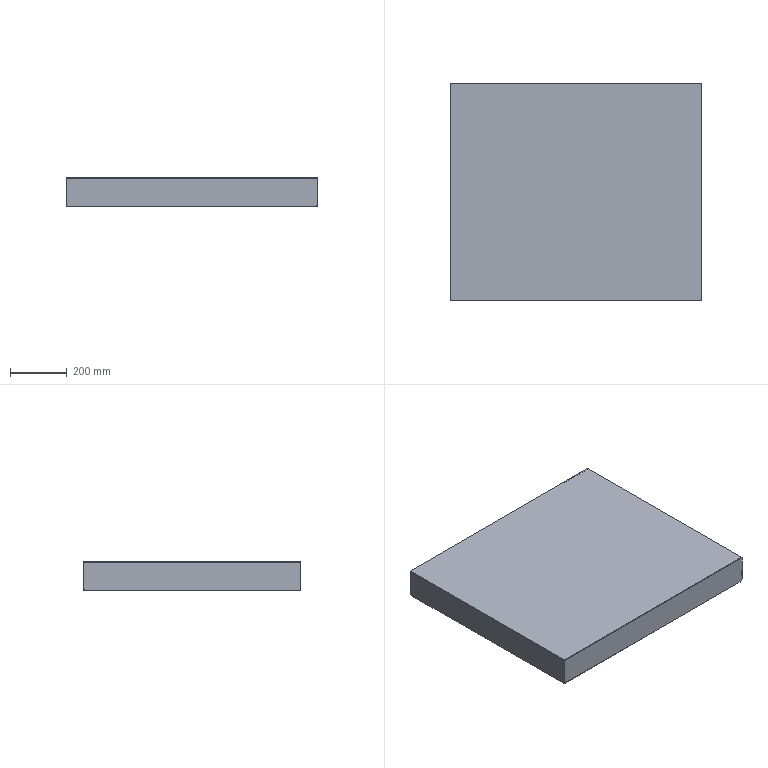Part | STEP file | PN_0047 checkered steel plate 3_Default<As Machined> | 3 solids | 23 faces | box 891 x 771 x 103 mm | volume 2594390 mm3 | plane 20 | cylinder 3 | commonest cylinder face diameters 20 x3
STEP:
#1=CARTESIAN_POINT('',(0.,0.,0.));
#2=DIRECTION('',(0.,0.,1.));
#3=DIRECTION('',(1.,0.,0.));
#4=AXIS2_PLACEMENT_3D('',#1,#2,#3);
#5=CARTESIAN_POINT('',(445.5,-385.5,0.));
#6=VERTEX_POINT('',#5);
#7=CARTESIAN_POINT('',(445.5,385.5,0.));
#8=VERTEX_POINT('',#7);
#9=CARTESIAN_POINT('',(445.5,385.5,0.));
#10=DIRECTION('',(0.,1.,0.));
#11=VECTOR('',#10,1.);
#12=LINE('',#9,#11);
#13=CARTESIAN_POINT('',(445.5,385.5,-3.));
#14=DIRECTION('',(1.,0.,0.));
#15=DIRECTION('',(0.,0.,-1.));
#16=AXIS2_PLACEMENT_3D('',#13,#14,#15);
#17=PLANE('',#16);
#18=CARTESIAN_POINT('',(-3.,0.));
#19=DIRECTION('',(0.,1.));
#20=VECTOR('',#19,1.);
#21=LINE('',#18,#20);
#22=(GEOMETRIC_REPRESENTATION_CONTEXT(2)PARAMETRIC_REPRESENTATION_CONTEXT()REPRESENTATION_CONTEXT('',''));
#23=DEFINITIONAL_REPRESENTATION('',(#21),#22);
#24=PCURVE('',#17,#23);
#25=CARTESIAN_POINT('',(0.,0.,0.));
#26=DIRECTION('',(0.,0.,1.));
#27=DIRECTION('',(1.,0.,0.));
#28=AXIS2_PLACEMENT_3D('',#25,#26,#27);
#29=PLANE('',#28);
#30=CARTESIAN_POINT('',(445.5,385.5));
#31=DIRECTION('',(0.,1.));
#32=VECTOR('',#31,1.);
#33=LINE('',#30,#32);
#34=(GEOMETRIC_REPRESENTATION_CONTEXT(2)PARAMETRIC_REPRESENTATION_CONTEXT()REPRESENTATION_CONTEXT('',''));
#35=DEFINITIONAL_REPRESENTATION('',(#33),#34);
#36=PCURVE('',#29,#35);
#37=SURFACE_CURVE('',#12,(#24,#36),.PCURVE_S1.);
#38=EDGE_CURVE('',#6,#8,#37,.T.);
#39=ORIENTED_EDGE('',*,*,#38,.F.);
#40=CARTESIAN_POINT('',(445.5,-385.5,-3.));
#41=VERTEX_POINT('',#40);
#42=CARTESIAN_POINT('',(445.5,-385.5,-3.));
#43=DIRECTION('',(0.,0.,1.));
#44=VECTOR('',#43,1.);
#45=LINE('',#42,#44);
#46=CARTESIAN_POINT('',(0.,-771.));
#47=DIRECTION('',(-1.,0.));
#48=VECTOR('',#47,1.);
#49=LINE('',#46,#48);
#50=(GEOMETRIC_REPRESENTATION_CONTEXT(2)PARAMETRIC_REPRESENTATION_CONTEXT()REPRESENTATION_CONTEXT('',''));
#51=DEFINITIONAL_REPRESENTATION('',(#49),#50);
#52=PCURVE('',#17,#51);
#53=CARTESIAN_POINT('',(-445.5,-385.5,-3.));
#54=DIRECTION('',(0.,-1.,0.));
#55=DIRECTION('',(0.,0.,-1.));
#56=AXIS2_PLACEMENT_3D('',#53,#54,#55);
#57=PLANE('',#56);
#58=CARTESIAN_POINT('',(0.,891.));
#59=DIRECTION('',(-1.,0.));
#60=VECTOR('',#59,1.);
#61=LINE('',#58,#60);
#62=(GEOMETRIC_REPRESENTATION_CONTEXT(2)PARAMETRIC_REPRESENTATION_CONTEXT()REPRESENTATION_CONTEXT('',''));
#63=DEFINITIONAL_REPRESENTATION('',(#61),#62);
#64=PCURVE('',#57,#63);
#65=SURFACE_CURVE('',#45,(#52,#64),.PCURVE_S1.);
#66=EDGE_CURVE('',#41,#6,#65,.T.);
#67=ORIENTED_EDGE('',*,*,#66,.F.);
#68=CARTESIAN_POINT('',(445.5,385.5,-3.));
#69=VERTEX_POINT('',#68);
#70=CARTESIAN_POINT('',(445.5,385.5,-3.));
#71=DIRECTION('',(0.,1.,0.));
#72=VECTOR('',#71,1.);
#73=LINE('',#70,#72);
#74=CARTESIAN_POINT('',(0.,0.));
#75=DIRECTION('',(0.,1.));
#76=VECTOR('',#75,1.);
#77=LINE('',#74,#76);
#78=(GEOMETRIC_REPRESENTATION_CONTEXT(2)PARAMETRIC_REPRESENTATION_CONTEXT()REPRESENTATION_CONTEXT('',''));
#79=DEFINITIONAL_REPRESENTATION('',(#77),#78);
#80=PCURVE('',#17,#79);
#81=CARTESIAN_POINT('',(0.,0.,-3.));
#82=DIRECTION('',(0.,0.,1.));
#83=DIRECTION('',(1.,0.,0.));
#84=AXIS2_PLACEMENT_3D('',#81,#82,#83);
#85=PLANE('',#84);
#86=CARTESIAN_POINT('',(445.5,385.5));
#87=DIRECTION('',(0.,1.));
#88=VECTOR('',#87,1.);
#89=LINE('',#86,#88);
#90=(GEOMETRIC_REPRESENTATION_CONTEXT(2)PARAMETRIC_REPRESENTATION_CONTEXT()REPRESENTATION_CONTEXT('',''));
#91=DEFINITIONAL_REPRESENTATION('',(#89),#90);
#92=PCURVE('',#85,#91);
#93=SURFACE_CURVE('',#73,(#80,#92),.PCURVE_S1.);
#94=EDGE_CURVE('',#41,#69,#93,.T.);
#95=ORIENTED_EDGE('',*,*,#94,.T.);
#96=CARTESIAN_POINT('',(445.5,385.5,-3.));
#97=DIRECTION('',(0.,0.,1.));
#98=VECTOR('',#97,1.);
#99=LINE('',#96,#98);
#100=CARTESIAN_POINT('',(0.,0.));
#101=DIRECTION('',(-1.,0.));
#102=VECTOR('',#101,1.);
#103=LINE('',#100,#102);
#104=(GEOMETRIC_REPRESENTATION_CONTEXT(2)PARAMETRIC_REPRESENTATION_CONTEXT()REPRESENTATION_CONTEXT('',''));
#105=DEFINITIONAL_REPRESENTATION('',(#103),#104);
#106=PCURVE('',#17,#105);
#107=CARTESIAN_POINT('',(-445.5,385.5,-3.));
#108=DIRECTION('',(0.,1.,0.));
#109=DIRECTION('',(0.,0.,1.));
#110=AXIS2_PLACEMENT_3D('',#107,#108,#109);
#111=PLANE('',#110);
#112=CARTESIAN_POINT('',(0.,891.));
#113=DIRECTION('',(1.,0.));
#114=VECTOR('',#113,1.);
#115=LINE('',#112,#114);
#116=(GEOMETRIC_REPRESENTATION_CONTEXT(2)PARAMETRIC_REPRESENTATION_CONTEXT()REPRESENTATION_CONTEXT('',''));
#117=DEFINITIONAL_REPRESENTATION('',(#115),#116);
#118=PCURVE('',#111,#117);
#119=SURFACE_CURVE('',#99,(#106,#118),.PCURVE_S1.);
#120=EDGE_CURVE('',#69,#8,#119,.T.);
#121=ORIENTED_EDGE('',*,*,#120,.T.);
#122=EDGE_LOOP('',(#39,#67,#95,#121));
#123=FACE_BOUND('',#122,.T.);
#124=ADVANCED_FACE('',(#123),#17,.T.);
#125=CARTESIAN_POINT('',(-445.5,-385.5,0.));
#126=VERTEX_POINT('',#125);
#127=CARTESIAN_POINT('',(-445.5,-385.5,0.));
#128=DIRECTION('',(1.,0.,0.));
#129=VECTOR('',#128,1.);
#130=LINE('',#127,#129);
#131=CARTESIAN_POINT('',(-3.,0.));
#132=DIRECTION('',(0.,1.));
#133=VECTOR('',#132,1.);
#134=LINE('',#131,#133);
#135=(GEOMETRIC_REPRESENTATION_CONTEXT(2)PARAMETRIC_REPRESENTATION_CONTEXT()REPRESENTATION_CONTEXT('',''));
#136=DEFINITIONAL_REPRESENTATION('',(#134),#135);
#137=PCURVE('',#57,#136);
#138=CARTESIAN_POINT('',(-445.5,-385.5));
#139=DIRECTION('',(1.,0.));
#140=VECTOR('',#139,1.);
#141=LINE('',#138,#140);
#142=(GEOMETRIC_REPRESENTATION_CONTEXT(2)PARAMETRIC_REPRESENTATION_CONTEXT()REPRESENTATION_CONTEXT('',''));
#143=DEFINITIONAL_REPRESENTATION('',(#141),#142);
#144=PCURVE('',#29,#143);
#145=SURFACE_CURVE('',#130,(#137,#144),.PCURVE_S1.);
#146=EDGE_CURVE('',#126,#6,#145,.T.);
#147=ORIENTED_EDGE('',*,*,#146,.F.);
#148=CARTESIAN_POINT('',(-445.5,-385.5,-3.));
#149=VERTEX_POINT('',#148);
#150=CARTESIAN_POINT('',(-445.5,-385.5,-3.));
#151=DIRECTION('',(0.,0.,1.));
#152=VECTOR('',#151,1.);
#153=LINE('',#150,#152);
#154=CARTESIAN_POINT('',(0.,0.));
#155=DIRECTION('',(-1.,0.));
#156=VECTOR('',#155,1.);
#157=LINE('',#154,#156);
#158=(GEOMETRIC_REPRESENTATION_CONTEXT(2)PARAMETRIC_REPRESENTATION_CONTEXT()REPRESENTATION_CONTEXT('',''));
#159=DEFINITIONAL_REPRESENTATION('',(#157),#158);
#160=PCURVE('',#57,#159);
#161=CARTESIAN_POINT('',(-445.5,385.5,-3.));
#162=DIRECTION('',(-1.,0.,0.));
#163=DIRECTION('',(0.,0.,1.));
#164=AXIS2_PLACEMENT_3D('',#161,#162,#163);
#165=PLANE('',#164);
#166=CARTESIAN_POINT('',(0.,-771.));
#167=DIRECTION('',(1.,0.));
#168=VECTOR('',#167,1.);
#169=LINE('',#166,#168);
#170=(GEOMETRIC_REPRESENTATION_CONTEXT(2)PARAMETRIC_REPRESENTATION_CONTEXT()REPRESENTATION_CONTEXT('',''));
#171=DEFINITIONAL_REPRESENTATION('',(#169),#170);
#172=PCURVE('',#165,#171);
#173=SURFACE_CURVE('',#153,(#160,#172),.PCURVE_S1.);
#174=EDGE_CURVE('',#149,#126,#173,.T.);
#175=ORIENTED_EDGE('',*,*,#174,.F.);
#176=CARTESIAN_POINT('',(-445.5,-385.5,-3.));
#177=DIRECTION('',(1.,0.,0.));
#178=VECTOR('',#177,1.);
#179=LINE('',#176,#178);
#180=CARTESIAN_POINT('',(0.,0.));
#181=DIRECTION('',(0.,1.));
#182=VECTOR('',#181,1.);
#183=LINE('',#180,#182);
#184=(GEOMETRIC_REPRESENTATION_CONTEXT(2)PARAMETRIC_REPRESENTATION_CONTEXT()REPRESENTATION_CONTEXT('',''));
#185=DEFINITIONAL_REPRESENTATION('',(#183),#184);
#186=PCURVE('',#57,#185);
#187=CARTESIAN_POINT('',(-445.5,-385.5));
#188=DIRECTION('',(1.,0.));
#189=VECTOR('',#188,1.);
#190=LINE('',#187,#189);
#191=(GEOMETRIC_REPRESENTATION_CONTEXT(2)PARAMETRIC_REPRESENTATION_CONTEXT()REPRESENTATION_CONTEXT('',''));
#192=DEFINITIONAL_REPRESENTATION('',(#190),#191);
#193=PCURVE('',#85,#192);
#194=SURFACE_CURVE('',#179,(#186,#193),.PCURVE_S1.);
#195=EDGE_CURVE('',#149,#41,#194,.T.);
#196=ORIENTED_EDGE('',*,*,#195,.T.);
#197=ORIENTED_EDGE('',*,*,#66,.T.);
#198=EDGE_LOOP('',(#147,#175,#196,#197));
#199=FACE_BOUND('',#198,.T.);
#200=ADVANCED_FACE('',(#199),#57,.T.);
#201=CARTESIAN_POINT('',(-445.5,385.5,0.));
#202=VERTEX_POINT('',#201);
#203=CARTESIAN_POINT('',(-445.5,385.5,0.));
#204=DIRECTION('',(0.,-1.,0.));
#205=VECTOR('',#204,1.);
#206=LINE('',#203,#205);
#207=CARTESIAN_POINT('',(3.,0.));
#208=DIRECTION('',(0.,-1.));
#209=VECTOR('',#208,1.);
#210=LINE('',#207,#209);
#211=(GEOMETRIC_REPRESENTATION_CONTEXT(2)PARAMETRIC_REPRESENTATION_CONTEXT()REPRESENTATION_CONTEXT('',''));
#212=DEFINITIONAL_REPRESENTATION('',(#210),#211);
#213=PCURVE('',#165,#212);
#214=CARTESIAN_POINT('',(-445.5,385.5));
#215=DIRECTION('',(0.,-1.));
#216=VECTOR('',#215,1.);
#217=LINE('',#214,#216);
#218=(GEOMETRIC_REPRESENTATION_CONTEXT(2)PARAMETRIC_REPRESENTATION_CONTEXT()REPRESENTATION_CONTEXT('',''));
#219=DEFINITIONAL_REPRESENTATION('',(#217),#218);
#220=PCURVE('',#29,#219);
#221=SURFACE_CURVE('',#206,(#213,#220),.PCURVE_S1.);
#222=EDGE_CURVE('',#202,#126,#221,.T.);
#223=ORIENTED_EDGE('',*,*,#222,.F.);
#224=CARTESIAN_POINT('',(-445.5,385.5,-3.));
#225=VERTEX_POINT('',#224);
#226=CARTESIAN_POINT('',(-445.5,385.5,-3.));
#227=DIRECTION('',(0.,0.,1.));
#228=VECTOR('',#227,1.);
#229=LINE('',#226,#228);
#230=CARTESIAN_POINT('',(0.,0.));
#231=DIRECTION('',(1.,0.));
#232=VECTOR('',#231,1.);
#233=LINE('',#230,#232);
#234=(GEOMETRIC_REPRESENTATION_CONTEXT(2)PARAMETRIC_REPRESENTATION_CONTEXT()REPRESENTATION_CONTEXT('',''));
#235=DEFINITIONAL_REPRESENTATION('',(#233),#234);
#236=PCURVE('',#165,#235);
#237=CARTESIAN_POINT('',(0.,0.));
#238=DIRECTION('',(1.,0.));
#239=VECTOR('',#238,1.);
#240=LINE('',#237,#239);
#241=(GEOMETRIC_REPRESENTATION_CONTEXT(2)PARAMETRIC_REPRESENTATION_CONTEXT()REPRESENTATION_CONTEXT('',''));
#242=DEFINITIONAL_REPRESENTATION('',(#240),#241);
#243=PCURVE('',#111,#242);
#244=SURFACE_CURVE('',#229,(#236,#243),.PCURVE_S1.);
#245=EDGE_CURVE('',#225,#202,#244,.T.);
#246=ORIENTED_EDGE('',*,*,#245,.F.);
#247=CARTESIAN_POINT('',(-445.5,385.5,-3.));
#248=DIRECTION('',(0.,-1.,0.));
#249=VECTOR('',#248,1.);
#250=LINE('',#247,#249);
#251=CARTESIAN_POINT('',(0.,0.));
#252=DIRECTION('',(0.,-1.));
#253=VECTOR('',#252,1.);
#254=LINE('',#251,#253);
#255=(GEOMETRIC_REPRESENTATION_CONTEXT(2)PARAMETRIC_REPRESENTATION_CONTEXT()REPRESENTATION_CONTEXT('',''));
#256=DEFINITIONAL_REPRESENTATION('',(#254),#255);
#257=PCURVE('',#165,#256);
#258=CARTESIAN_POINT('',(-445.5,385.5));
#259=DIRECTION('',(0.,-1.));
#260=VECTOR('',#259,1.);
#261=LINE('',#258,#260);
#262=(GEOMETRIC_REPRESENTATION_CONTEXT(2)PARAMETRIC_REPRESENTATION_CONTEXT()REPRESENTATION_CONTEXT('',''));
#263=DEFINITIONAL_REPRESENTATION('',(#261),#262);
#264=PCURVE('',#85,#263);
#265=SURFACE_CURVE('',#250,(#257,#264),.PCURVE_S1.);
#266=EDGE_CURVE('',#225,#149,#265,.T.);
#267=ORIENTED_EDGE('',*,*,#266,.T.);
#268=ORIENTED_EDGE('',*,*,#174,.T.);
#269=EDGE_LOOP('',(#223,#246,#267,#268));
#270=FACE_BOUND('',#269,.T.);
#271=ADVANCED_FACE('',(#270),#165,.T.);
#272=CARTESIAN_POINT('',(-445.5,385.5,0.));
#273=DIRECTION('',(-1.,0.,0.));
#274=VECTOR('',#273,1.);
#275=LINE('',#272,#274);
#276=CARTESIAN_POINT('',(3.,0.));
#277=DIRECTION('',(0.,-1.));
#278=VECTOR('',#277,1.);
#279=LINE('',#276,#278);
#280=(GEOMETRIC_REPRESENTATION_CONTEXT(2)PARAMETRIC_REPRESENTATION_CONTEXT()REPRESENTATION_CONTEXT('',''));
#281=DEFINITIONAL_REPRESENTATION('',(#279),#280);
#282=PCURVE('',#111,#281);
#283=CARTESIAN_POINT('',(-445.5,385.5));
#284=DIRECTION('',(-1.,0.));
#285=VECTOR('',#284,1.);
#286=LINE('',#283,#285);
#287=(GEOMETRIC_REPRESENTATION_CONTEXT(2)PARAMETRIC_REPRESENTATION_CONTEXT()REPRESENTATION_CONTEXT('',''));
#288=DEFINITIONAL_REPRESENTATION('',(#286),#287);
#289=PCURVE('',#29,#288);
#290=SURFACE_CURVE('',#275,(#282,#289),.PCURVE_S1.);
#291=EDGE_CURVE('',#8,#202,#290,.T.);
#292=ORIENTED_EDGE('',*,*,#291,.F.);
#293=ORIENTED_EDGE('',*,*,#120,.F.);
#294=CARTESIAN_POINT('',(-445.5,385.5,-3.));
#295=DIRECTION('',(-1.,0.,0.));
#296=VECTOR('',#295,1.);
#297=LINE('',#294,#296);
#298=CARTESIAN_POINT('',(0.,0.));
#299=DIRECTION('',(0.,-1.));
#300=VECTOR('',#299,1.);
#301=LINE('',#298,#300);
#302=(GEOMETRIC_REPRESENTATION_CONTEXT(2)PARAMETRIC_REPRESENTATION_CONTEXT()REPRESENTATION_CONTEXT('',''));
#303=DEFINITIONAL_REPRESENTATION('',(#301),#302);
#304=PCURVE('',#111,#303);
#305=CARTESIAN_POINT('',(-445.5,385.5));
#306=DIRECTION('',(-1.,0.));
#307=VECTOR('',#306,1.);
#308=LINE('',#305,#307);
#309=(GEOMETRIC_REPRESENTATION_CONTEXT(2)PARAMETRIC_REPRESENTATION_CONTEXT()REPRESENTATION_CONTEXT('',''));
#310=DEFINITIONAL_REPRESENTATION('',(#308),#309);
#311=PCURVE('',#85,#310);
#312=SURFACE_CURVE('',#297,(#304,#311),.PCURVE_S1.);
#313=EDGE_CURVE('',#69,#225,#312,.T.);
#314=ORIENTED_EDGE('',*,*,#313,.T.);
#315=ORIENTED_EDGE('',*,*,#245,.T.);
#316=EDGE_LOOP('',(#292,#293,#314,#315));
#317=FACE_BOUND('',#316,.T.);
#318=ADVANCED_FACE('',(#317),#111,.T.);
#319=ORIENTED_EDGE('',*,*,#94,.F.);
#320=ORIENTED_EDGE('',*,*,#195,.F.);
#321=ORIENTED_EDGE('',*,*,#266,.F.);
#322=ORIENTED_EDGE('',*,*,#313,.F.);
#323=EDGE_LOOP('',(#319,#320,#321,#322));
#324=FACE_BOUND('',#323,.T.);
#325=ADVANCED_FACE('',(#324),#85,.F.);
#326=ORIENTED_EDGE('',*,*,#38,.T.);
#327=ORIENTED_EDGE('',*,*,#291,.T.);
#328=ORIENTED_EDGE('',*,*,#222,.T.);
#329=ORIENTED_EDGE('',*,*,#146,.T.);
#330=EDGE_LOOP('',(#326,#327,#328,#329));
#331=FACE_BOUND('',#330,.T.);
#332=ADVANCED_FACE('',(#331),#29,.T.);
#333=CLOSED_SHELL('',(#124,#200,#271,#318,#325,#332));
#334=MANIFOLD_SOLID_BREP('',#333);
#335=CARTESIAN_POINT('',(-445.5,-385.5,-103.));
#336=VERTEX_POINT('',#335);
#337=CARTESIAN_POINT('',(435.5,-385.5,-103.));
#338=VERTEX_POINT('',#337);
#339=CARTESIAN_POINT('',(-445.5,-385.5,-103.));
#340=DIRECTION('',(1.,0.,0.));
#341=VECTOR('',#340,1.);
#342=LINE('',#339,#341);
#343=CARTESIAN_POINT('',(-445.5,-385.5,-103.));
#344=DIRECTION('',(0.,-1.,0.));
#345=DIRECTION('',(0.,0.,-1.));
#346=AXIS2_PLACEMENT_3D('',#343,#344,#345);
#347=PLANE('',#346);
#348=CARTESIAN_POINT('',(0.,0.));
#349=DIRECTION('',(0.,1.));
#350=VECTOR('',#349,1.);
#351=LINE('',#348,#350);
#352=(GEOMETRIC_REPRESENTATION_CONTEXT(2)PARAMETRIC_REPRESENTATION_CONTEXT()REPRESENTATION_CONTEXT('',''));
#353=DEFINITIONAL_REPRESENTATION('',(#351),#352);
#354=PCURVE('',#347,#353);
#355=CARTESIAN_POINT('',(0.,0.,-103.));
#356=DIRECTION('',(0.,0.,-1.));
#357=DIRECTION('',(-1.,0.,0.));
#358=AXIS2_PLACEMENT_3D('',#355,#356,#357);
#359=PLANE('',#358);
#360=CARTESIAN_POINT('',(445.5,-385.5));
#361=DIRECTION('',(-1.,0.));
#362=VECTOR('',#361,1.);
#363=LINE('',#360,#362);
#364=(GEOMETRIC_REPRESENTATION_CONTEXT(2)PARAMETRIC_REPRESENTATION_CONTEXT()REPRESENTATION_CONTEXT('',''));
#365=DEFINITIONAL_REPRESENTATION('',(#363),#364);
#366=PCURVE('',#359,#365);
#367=SURFACE_CURVE('',#342,(#354,#366),.PCURVE_S1.);
#368=EDGE_CURVE('',#336,#338,#367,.T.);
#369=ORIENTED_EDGE('',*,*,#368,.T.);
#370=CARTESIAN_POINT('',(445.5,-385.5,-93.));
#371=VERTEX_POINT('',#370);
#372=CARTESIAN_POINT('',(435.5,-385.5,-93.));
#373=DIRECTION('',(0.,-1.,0.));
#374=DIRECTION('',(0.,0.,-1.));
#375=AXIS2_PLACEMENT_3D('',#372,#373,#374);
#376=CIRCLE('',#375,10.);
#377=CARTESIAN_POINT('',(-10.,881.));
#378=DIRECTION('',(1.,0.));
#379=AXIS2_PLACEMENT_2D('',#377,#378);
#380=CIRCLE('',#379,10.);
#381=(GEOMETRIC_REPRESENTATION_CONTEXT(2)PARAMETRIC_REPRESENTATION_CONTEXT()REPRESENTATION_CONTEXT('',''));
#382=DEFINITIONAL_REPRESENTATION('',(#380),#381);
#383=PCURVE('',#347,#382);
#384=CARTESIAN_POINT('',(435.5,0.,-93.));
#385=DIRECTION('',(0.,1.,0.));
#386=DIRECTION('',(0.,0.,1.));
#387=AXIS2_PLACEMENT_3D('',#384,#385,#386);
#388=CYLINDRICAL_SURFACE('',#387,10.);
#389=CARTESIAN_POINT('',(3.142,-385.5));
#390=DIRECTION('',(-1.,0.));
#391=VECTOR('',#390,1.);
#392=LINE('',#389,#391);
#393=(GEOMETRIC_REPRESENTATION_CONTEXT(2)PARAMETRIC_REPRESENTATION_CONTEXT()REPRESENTATION_CONTEXT('',''));
#394=DEFINITIONAL_REPRESENTATION('',(#392),#393);
#395=PCURVE('',#388,#394);
#396=SURFACE_CURVE('',#376,(#383,#395),.PCURVE_S1.);
#397=EDGE_CURVE('',#338,#371,#396,.T.);
#398=ORIENTED_EDGE('',*,*,#397,.T.);
#399=CARTESIAN_POINT('',(445.5,-385.5,-3.));
#400=VERTEX_POINT('',#399);
#401=CARTESIAN_POINT('',(445.5,-385.5,-103.));
#402=DIRECTION('',(0.,0.,1.));
#403=VECTOR('',#402,1.);
#404=LINE('',#401,#403);
#405=CARTESIAN_POINT('',(0.,891.));
#406=DIRECTION('',(-1.,0.));
#407=VECTOR('',#406,1.);
#408=LINE('',#405,#407);
#409=(GEOMETRIC_REPRESENTATION_CONTEXT(2)PARAMETRIC_REPRESENTATION_CONTEXT()REPRESENTATION_CONTEXT('',''));
#410=DEFINITIONAL_REPRESENTATION('',(#408),#409);
#411=PCURVE('',#347,#410);
#412=CARTESIAN_POINT('',(445.5,-382.5,-103.));
#413=DIRECTION('',(-1.,0.,0.));
#414=DIRECTION('',(0.,0.,1.));
#415=AXIS2_PLACEMENT_3D('',#412,#413,#414);
#416=PLANE('',#415);
#417=CARTESIAN_POINT('',(0.,-3.));
#418=DIRECTION('',(1.,0.));
#419=VECTOR('',#418,1.);
#420=LINE('',#417,#419);
#421=(GEOMETRIC_REPRESENTATION_CONTEXT(2)PARAMETRIC_REPRESENTATION_CONTEXT()REPRESENTATION_CONTEXT('',''));
#422=DEFINITIONAL_REPRESENTATION('',(#420),#421);
#423=PCURVE('',#416,#422);
#424=SURFACE_CURVE('',#404,(#411,#423),.PCURVE_S1.);
#425=EDGE_CURVE('',#371,#400,#424,.T.);
#426=ORIENTED_EDGE('',*,*,#425,.T.);
#427=CARTESIAN_POINT('',(-445.5,-385.5,-3.));
#428=VERTEX_POINT('',#427);
#429=CARTESIAN_POINT('',(-445.5,-385.5,-3.));
#430=DIRECTION('',(1.,0.,0.));
#431=VECTOR('',#430,1.);
#432=LINE('',#429,#431);
#433=CARTESIAN_POINT('',(-100.,0.));
#434=DIRECTION('',(0.,1.));
#435=VECTOR('',#434,1.);
#436=LINE('',#433,#435);
#437=(GEOMETRIC_REPRESENTATION_CONTEXT(2)PARAMETRIC_REPRESENTATION_CONTEXT()REPRESENTATION_CONTEXT('',''));
#438=DEFINITIONAL_REPRESENTATION('',(#436),#437);
#439=PCURVE('',#347,#438);
#440=CARTESIAN_POINT('',(0.,0.,-3.));
#441=DIRECTION('',(0.,0.,-1.));
#442=DIRECTION('',(-1.,0.,0.));
#443=AXIS2_PLACEMENT_3D('',#440,#441,#442);
#444=PLANE('',#443);
#445=CARTESIAN_POINT('',(445.5,-385.5));
#446=DIRECTION('',(-1.,0.));
#447=VECTOR('',#446,1.);
#448=LINE('',#445,#447);
#449=(GEOMETRIC_REPRESENTATION_CONTEXT(2)PARAMETRIC_REPRESENTATION_CONTEXT()REPRESENTATION_CONTEXT('',''));
#450=DEFINITIONAL_REPRESENTATION('',(#448),#449);
#451=PCURVE('',#444,#450);
#452=SURFACE_CURVE('',#432,(#439,#451),.PCURVE_S1.);
#453=EDGE_CURVE('',#428,#400,#452,.T.);
#454=ORIENTED_EDGE('',*,*,#453,.F.);
#455=CARTESIAN_POINT('',(-445.5,-385.5,-103.));
#456=DIRECTION('',(0.,0.,1.));
#457=VECTOR('',#456,1.);
#458=LINE('',#455,#457);
#459=CARTESIAN_POINT('',(0.,0.));
#460=DIRECTION('',(-1.,0.));
#461=VECTOR('',#460,1.);
#462=LINE('',#459,#461);
#463=(GEOMETRIC_REPRESENTATION_CONTEXT(2)PARAMETRIC_REPRESENTATION_CONTEXT()REPRESENTATION_CONTEXT('',''));
#464=DEFINITIONAL_REPRESENTATION('',(#462),#463);
#465=PCURVE('',#347,#464);
#466=CARTESIAN_POINT('',(-445.5,385.5,-103.));
#467=DIRECTION('',(-1.,0.,0.));
#468=DIRECTION('',(0.,0.,1.));
#469=AXIS2_PLACEMENT_3D('',#466,#467,#468);
#470=PLANE('',#469);
#471=CARTESIAN_POINT('',(0.,-771.));
#472=DIRECTION('',(1.,0.));
#473=VECTOR('',#472,1.);
#474=LINE('',#471,#473);
#475=(GEOMETRIC_REPRESENTATION_CONTEXT(2)PARAMETRIC_REPRESENTATION_CONTEXT()REPRESENTATION_CONTEXT('',''));
#476=DEFINITIONAL_REPRESENTATION('',(#474),#475);
#477=PCURVE('',#470,#476);
#478=SURFACE_CURVE('',#458,(#465,#477),.PCURVE_S1.);
#479=EDGE_CURVE('',#336,#428,#478,.T.);
#480=ORIENTED_EDGE('',*,*,#479,.F.);
#481=EDGE_LOOP('',(#369,#398,#426,#454,#480));
#482=FACE_BOUND('',#481,.T.);
#483=ADVANCED_FACE('',(#482),#347,.T.);
#484=CARTESIAN_POINT('',(-445.5,385.5,-93.));
#485=VERTEX_POINT('',#484);
#486=CARTESIAN_POINT('',(-445.5,385.5,-3.));
#487=VERTEX_POINT('',#486);
#488=CARTESIAN_POINT('',(-445.5,385.5,-103.));
#489=DIRECTION('',(0.,0.,1.));
#490=VECTOR('',#489,1.);
#491=LINE('',#488,#490);
#492=CARTESIAN_POINT('',(0.,0.));
#493=DIRECTION('',(1.,0.));
#494=VECTOR('',#493,1.);
#495=LINE('',#492,#494);
#496=(GEOMETRIC_REPRESENTATION_CONTEXT(2)PARAMETRIC_REPRESENTATION_CONTEXT()REPRESENTATION_CONTEXT('',''));
#497=DEFINITIONAL_REPRESENTATION('',(#495),#496);
#498=PCURVE('',#470,#497);
#499=CARTESIAN_POINT('',(-445.5,385.5,-103.));
#500=DIRECTION('',(0.,-1.,0.));
#501=DIRECTION('',(0.,0.,-1.));
#502=AXIS2_PLACEMENT_3D('',#499,#500,#501);
#503=PLANE('',#502);
#504=CARTESIAN_POINT('',(0.,0.));
#505=DIRECTION('',(-1.,0.));
#506=VECTOR('',#505,1.);
#507=LINE('',#504,#506);
#508=(GEOMETRIC_REPRESENTATION_CONTEXT(2)PARAMETRIC_REPRESENTATION_CONTEXT()REPRESENTATION_CONTEXT('',''));
#509=DEFINITIONAL_REPRESENTATION('',(#507),#508);
#510=PCURVE('',#503,#509);
#511=SURFACE_CURVE('',#491,(#498,#510),.PCURVE_S1.);
#512=EDGE_CURVE('',#485,#487,#511,.T.);
#513=ORIENTED_EDGE('',*,*,#512,.F.);
#514=CARTESIAN_POINT('',(-445.5,375.5,-103.));
#515=VERTEX_POINT('',#514);
#516=CARTESIAN_POINT('',(-445.5,375.5,-93.));
#517=DIRECTION('',(-1.,0.,0.));
#518=DIRECTION('',(0.,0.,1.));
#519=AXIS2_PLACEMENT_3D('',#516,#517,#518);
#520=CIRCLE('',#519,10.);
#521=CARTESIAN_POINT('',(10.,-10.));
#522=DIRECTION('',(1.,0.));
#523=AXIS2_PLACEMENT_2D('',#521,#522);
#524=CIRCLE('',#523,10.);
#525=(GEOMETRIC_REPRESENTATION_CONTEXT(2)PARAMETRIC_REPRESENTATION_CONTEXT()REPRESENTATION_CONTEXT('',''));
#526=DEFINITIONAL_REPRESENTATION('',(#524),#525);
#527=PCURVE('',#470,#526);
#528=CARTESIAN_POINT('',(0.,375.5,-93.));
#529=DIRECTION('',(-1.,0.,0.));
#530=DIRECTION('',(0.,0.,1.));
#531=AXIS2_PLACEMENT_3D('',#528,#529,#530);
#532=CYLINDRICAL_SURFACE('',#531,10.);
#533=CARTESIAN_POINT('',(0.,445.5));
#534=DIRECTION('',(1.,0.));
#535=VECTOR('',#534,1.);
#536=LINE('',#533,#535);
#537=(GEOMETRIC_REPRESENTATION_CONTEXT(2)PARAMETRIC_REPRESENTATION_CONTEXT()REPRESENTATION_CONTEXT('',''));
#538=DEFINITIONAL_REPRESENTATION('',(#536),#537);
#539=PCURVE('',#532,#538);
#540=SURFACE_CURVE('',#520,(#527,#539),.PCURVE_S1.);
#541=EDGE_CURVE('',#485,#515,#540,.T.);
#542=ORIENTED_EDGE('',*,*,#541,.T.);
#543=CARTESIAN_POINT('',(-445.5,385.5,-103.));
#544=DIRECTION('',(0.,-1.,0.));
#545=VECTOR('',#544,1.);
#546=LINE('',#543,#545);
#547=CARTESIAN_POINT('',(0.,0.));
#548=DIRECTION('',(0.,-1.));
#549=VECTOR('',#548,1.);
#550=LINE('',#547,#549);
#551=(GEOMETRIC_REPRESENTATION_CONTEXT(2)PARAMETRIC_REPRESENTATION_CONTEXT()REPRESENTATION_CONTEXT('',''));
#552=DEFINITIONAL_REPRESENTATION('',(#550),#551);
#553=PCURVE('',#470,#552);
#554=CARTESIAN_POINT('',(445.5,385.5));
#555=DIRECTION('',(0.,-1.));
#556=VECTOR('',#555,1.);
#557=LINE('',#554,#556);
#558=(GEOMETRIC_REPRESENTATION_CONTEXT(2)PARAMETRIC_REPRESENTATION_CONTEXT()REPRESENTATION_CONTEXT('',''));
#559=DEFINITIONAL_REPRESENTATION('',(#557),#558);
#560=PCURVE('',#359,#559);
#561=SURFACE_CURVE('',#546,(#553,#560),.PCURVE_S1.);
#562=EDGE_CURVE('',#515,#336,#561,.T.);
#563=ORIENTED_EDGE('',*,*,#562,.T.);
#564=ORIENTED_EDGE('',*,*,#479,.T.);
#565=CARTESIAN_POINT('',(-445.5,385.5,-3.));
#566=DIRECTION('',(0.,-1.,0.));
#567=VECTOR('',#566,1.);
#568=LINE('',#565,#567);
#569=CARTESIAN_POINT('',(100.,0.));
#570=DIRECTION('',(0.,-1.));
#571=VECTOR('',#570,1.);
#572=LINE('',#569,#571);
#573=(GEOMETRIC_REPRESENTATION_CONTEXT(2)PARAMETRIC_REPRESENTATION_CONTEXT()REPRESENTATION_CONTEXT('',''));
#574=DEFINITIONAL_REPRESENTATION('',(#572),#573);
#575=PCURVE('',#470,#574);
#576=CARTESIAN_POINT('',(445.5,385.5));
#577=DIRECTION('',(0.,-1.));
#578=VECTOR('',#577,1.);
#579=LINE('',#576,#578);
#580=(GEOMETRIC_REPRESENTATION_CONTEXT(2)PARAMETRIC_REPRESENTATION_CONTEXT()REPRESENTATION_CONTEXT('',''));
#581=DEFINITIONAL_REPRESENTATION('',(#579),#580);
#582=PCURVE('',#444,#581);
#583=SURFACE_CURVE('',#568,(#575,#582),.PCURVE_S1.);
#584=EDGE_CURVE('',#487,#428,#583,.T.);
#585=ORIENTED_EDGE('',*,*,#584,.F.);
#586=EDGE_LOOP('',(#513,#542,#563,#564,#585));
#587=FACE_BOUND('',#586,.T.);
#588=ADVANCED_FACE('',(#587),#470,.T.);
#589=CARTESIAN_POINT('',(-442.5,385.5,-93.));
#590=VERTEX_POINT('',#589);
#591=CARTESIAN_POINT('',(-442.5,385.5,-3.));
#592=VERTEX_POINT('',#591);
#593=CARTESIAN_POINT('',(-442.5,385.5,-103.));
#594=DIRECTION('',(0.,0.,1.));
#595=VECTOR('',#594,1.);
#596=LINE('',#593,#595);
#597=CARTESIAN_POINT('',(0.,3.));
#598=DIRECTION('',(-1.,0.));
#599=VECTOR('',#598,1.);
#600=LINE('',#597,#599);
#601=(GEOMETRIC_REPRESENTATION_CONTEXT(2)PARAMETRIC_REPRESENTATION_CONTEXT()REPRESENTATION_CONTEXT('',''));
#602=DEFINITIONAL_REPRESENTATION('',(#600),#601);
#603=PCURVE('',#503,#602);
#604=CARTESIAN_POINT('',(-442.5,385.5,-103.));
#605=DIRECTION('',(-1.,0.,0.));
#606=DIRECTION('',(0.,0.,1.));
#607=AXIS2_PLACEMENT_3D('',#604,#605,#606);
#608=PLANE('',#607);
#609=CARTESIAN_POINT('',(0.,0.));
#610=DIRECTION('',(1.,0.));
#611=VECTOR('',#610,1.);
#612=LINE('',#609,#611);
#613=(GEOMETRIC_REPRESENTATION_CONTEXT(2)PARAMETRIC_REPRESENTATION_CONTEXT()REPRESENTATION_CONTEXT('',''));
#614=DEFINITIONAL_REPRESENTATION('',(#612),#613);
#615=PCURVE('',#608,#614);
#616=SURFACE_CURVE('',#596,(#603,#615),.PCURVE_S1.);
#617=EDGE_CURVE('',#590,#592,#616,.T.);
#618=ORIENTED_EDGE('',*,*,#617,.F.);
#619=CARTESIAN_POINT('',(-445.5,385.5,-93.));
#620=DIRECTION('',(-1.,0.,0.));
#621=VECTOR('',#620,1.);
#622=LINE('',#619,#621);
#623=CARTESIAN_POINT('',(-10.,0.));
#624=DIRECTION('',(0.,-1.));
#625=VECTOR('',#624,1.);
#626=LINE('',#623,#625);
#627=(GEOMETRIC_REPRESENTATION_CONTEXT(2)PARAMETRIC_REPRESENTATION_CONTEXT()REPRESENTATION_CONTEXT('',''));
#628=DEFINITIONAL_REPRESENTATION('',(#626),#627);
#629=PCURVE('',#503,#628);
#630=CARTESIAN_POINT('',(1.571,445.5));
#631=DIRECTION('',(0.,1.));
#632=VECTOR('',#631,1.);
#633=LINE('',#630,#632);
#634=(GEOMETRIC_REPRESENTATION_CONTEXT(2)PARAMETRIC_REPRESENTATION_CONTEXT()REPRESENTATION_CONTEXT('',''));
#635=DEFINITIONAL_REPRESENTATION('',(#633),#634);
#636=PCURVE('',#532,#635);
#637=SURFACE_CURVE('',#622,(#629,#636),.PCURVE_S1.);
#638=EDGE_CURVE('',#590,#485,#637,.T.);
#639=ORIENTED_EDGE('',*,*,#638,.T.);
#640=ORIENTED_EDGE('',*,*,#512,.T.);
#641=CARTESIAN_POINT('',(-445.5,385.5,-3.));
#642=DIRECTION('',(1.,0.,0.));
#643=VECTOR('',#642,1.);
#644=LINE('',#641,#643);
#645=CARTESIAN_POINT('',(-100.,0.));
#646=DIRECTION('',(0.,1.));
#647=VECTOR('',#646,1.);
#648=LINE('',#645,#647);
#649=(GEOMETRIC_REPRESENTATION_CONTEXT(2)PARAMETRIC_REPRESENTATION_CONTEXT()REPRESENTATION_CONTEXT('',''));
#650=DEFINITIONAL_REPRESENTATION('',(#648),#649);
#651=PCURVE('',#503,#650);
#652=CARTESIAN_POINT('',(445.5,385.5));
#653=DIRECTION('',(-1.,0.));
#654=VECTOR('',#653,1.);
#655=LINE('',#652,#654);
#656=(GEOMETRIC_REPRESENTATION_CONTEXT(2)PARAMETRIC_REPRESENTATION_CONTEXT()REPRESENTATION_CONTEXT('',''));
#657=DEFINITIONAL_REPRESENTATION('',(#655),#656);
#658=PCURVE('',#444,#657);
#659=SURFACE_CURVE('',#644,(#651,#658),.PCURVE_S1.);
#660=EDGE_CURVE('',#487,#592,#659,.T.);
#661=ORIENTED_EDGE('',*,*,#660,.T.);
#662=EDGE_LOOP('',(#618,#639,#640,#661));
#663=FACE_BOUND('',#662,.T.);
#664=ADVANCED_FACE('',(#663),#503,.F.);
#665=CARTESIAN_POINT('',(-442.5,375.5,-103.));
#666=VERTEX_POINT('',#665);
#667=CARTESIAN_POINT('',(-442.5,-382.5,-103.));
#668=VERTEX_POINT('',#667);
#669=CARTESIAN_POINT('',(-442.5,385.5,-103.));
#670=DIRECTION('',(0.,-1.,0.));
#671=VECTOR('',#670,1.);
#672=LINE('',#669,#671);
#673=CARTESIAN_POINT('',(0.,0.));
#674=DIRECTION('',(0.,-1.));
#675=VECTOR('',#674,1.);
#676=LINE('',#673,#675);
#677=(GEOMETRIC_REPRESENTATION_CONTEXT(2)PARAMETRIC_REPRESENTATION_CONTEXT()REPRESENTATION_CONTEXT('',''));
#678=DEFINITIONAL_REPRESENTATION('',(#676),#677);
#679=PCURVE('',#608,#678);
#680=CARTESIAN_POINT('',(442.5,385.5));
#681=DIRECTION('',(0.,-1.));
#682=VECTOR('',#681,1.);
#683=LINE('',#680,#682);
#684=(GEOMETRIC_REPRESENTATION_CONTEXT(2)PARAMETRIC_REPRESENTATION_CONTEXT()REPRESENTATION_CONTEXT('',''));
#685=DEFINITIONAL_REPRESENTATION('',(#683),#684);
#686=PCURVE('',#359,#685);
#687=SURFACE_CURVE('',#672,(#679,#686),.PCURVE_S1.);
#688=EDGE_CURVE('',#666,#668,#687,.T.);
#689=ORIENTED_EDGE('',*,*,#688,.F.);
#690=CARTESIAN_POINT('',(-442.5,375.5,-93.));
#691=DIRECTION('',(1.,0.,0.));
#692=DIRECTION('',(0.,0.,1.));
#693=AXIS2_PLACEMENT_3D('',#690,#691,#692);
#694=CIRCLE('',#693,10.);
#695=CARTESIAN_POINT('',(20.,-10.));
#696=CARTESIAN_POINT('',(20.,-27.321));
#697=CARTESIAN_POINT('',(5.,-18.66));
#698=CARTESIAN_POINT('',(-10.,-10.));
#699=CARTESIAN_POINT('',(5.,-1.34));
#700=CARTESIAN_POINT('',(20.,7.321));
#701=CARTESIAN_POINT('',(20.,-10.));
#702=(BOUNDED_CURVE()B_SPLINE_CURVE(2,(#695,#696,#697,#698,#699,#700,#701),.UNSPECIFIED.,.T.,.F.)B_SPLINE_CURVE_WITH_KNOTS((1,2,2,2,2,1),(-2.094,0.,2.094,4.189,6.283,8.378),.UNSPECIFIED.)CURVE()GEOMETRIC_REPRESENTATION_ITEM()RATIONAL_B_SPLINE_CURVE((1.,0.5,1.,0.5,1.,0.5,1.))REPRESENTATION_ITEM(''));
#703=(GEOMETRIC_REPRESENTATION_CONTEXT(2)PARAMETRIC_REPRESENTATION_CONTEXT()REPRESENTATION_CONTEXT('',''));
#704=DEFINITIONAL_REPRESENTATION('',(#702),#703);
#705=PCURVE('',#608,#704);
#706=CARTESIAN_POINT('',(6.283,442.5));
#707=DIRECTION('',(-1.,0.));
#708=VECTOR('',#707,1.);
#709=LINE('',#706,#708);
#710=(GEOMETRIC_REPRESENTATION_CONTEXT(2)PARAMETRIC_REPRESENTATION_CONTEXT()REPRESENTATION_CONTEXT('',''));
#711=DEFINITIONAL_REPRESENTATION('',(#709),#710);
#712=PCURVE('',#532,#711);
#713=SURFACE_CURVE('',#694,(#705,#712),.PCURVE_S1.);
#714=EDGE_CURVE('',#666,#590,#713,.T.);
#715=ORIENTED_EDGE('',*,*,#714,.T.);
#716=ORIENTED_EDGE('',*,*,#617,.T.);
#717=CARTESIAN_POINT('',(-442.5,-382.5,-3.));
#718=VERTEX_POINT('',#717);
#719=CARTESIAN_POINT('',(-442.5,385.5,-3.));
#720=DIRECTION('',(0.,-1.,0.));
#721=VECTOR('',#720,1.);
#722=LINE('',#719,#721);
#723=CARTESIAN_POINT('',(100.,0.));
#724=DIRECTION('',(0.,-1.));
#725=VECTOR('',#724,1.);
#726=LINE('',#723,#725);
#727=(GEOMETRIC_REPRESENTATION_CONTEXT(2)PARAMETRIC_REPRESENTATION_CONTEXT()REPRESENTATION_CONTEXT('',''));
#728=DEFINITIONAL_REPRESENTATION('',(#726),#727);
#729=PCURVE('',#608,#728);
#730=CARTESIAN_POINT('',(442.5,385.5));
#731=DIRECTION('',(0.,-1.));
#732=VECTOR('',#731,1.);
#733=LINE('',#730,#732);
#734=(GEOMETRIC_REPRESENTATION_CONTEXT(2)PARAMETRIC_REPRESENTATION_CONTEXT()REPRESENTATION_CONTEXT('',''));
#735=DEFINITIONAL_REPRESENTATION('',(#733),#734);
#736=PCURVE('',#444,#735);
#737=SURFACE_CURVE('',#722,(#729,#736),.PCURVE_S1.);
#738=EDGE_CURVE('',#592,#718,#737,.T.);
#739=ORIENTED_EDGE('',*,*,#738,.T.);
#740=CARTESIAN_POINT('',(-442.5,-382.5,-103.));
#741=DIRECTION('',(0.,0.,1.));
#742=VECTOR('',#741,1.);
#743=LINE('',#740,#742);
#744=CARTESIAN_POINT('',(0.,-768.));
#745=DIRECTION('',(1.,0.));
#746=VECTOR('',#745,1.);
#747=LINE('',#744,#746);
#748=(GEOMETRIC_REPRESENTATION_CONTEXT(2)PARAMETRIC_REPRESENTATION_CONTEXT()REPRESENTATION_CONTEXT('',''));
#749=DEFINITIONAL_REPRESENTATION('',(#747),#748);
#750=PCURVE('',#608,#749);
#751=CARTESIAN_POINT('',(-445.5,-382.5,-103.));
#752=DIRECTION('',(0.,-1.,0.));
#753=DIRECTION('',(0.,0.,-1.));
#754=AXIS2_PLACEMENT_3D('',#751,#752,#753);
#755=PLANE('',#754);
#756=CARTESIAN_POINT('',(0.,3.));
#757=DIRECTION('',(-1.,0.));
#758=VECTOR('',#757,1.);
#759=LINE('',#756,#758);
#760=(GEOMETRIC_REPRESENTATION_CONTEXT(2)PARAMETRIC_REPRESENTATION_CONTEXT()REPRESENTATION_CONTEXT('',''));
#761=DEFINITIONAL_REPRESENTATION('',(#759),#760);
#762=PCURVE('',#755,#761);
#763=SURFACE_CURVE('',#743,(#750,#762),.PCURVE_S1.);
#764=EDGE_CURVE('',#668,#718,#763,.T.);
#765=ORIENTED_EDGE('',*,*,#764,.F.);
#766=EDGE_LOOP('',(#689,#715,#716,#739,#765));
#767=FACE_BOUND('',#766,.T.);
#768=ADVANCED_FACE('',(#767),#608,.F.);
#769=CARTESIAN_POINT('',(445.5,-382.5,-93.));
#770=VERTEX_POINT('',#769);
#771=CARTESIAN_POINT('',(445.5,-382.5,-3.));
#772=VERTEX_POINT('',#771);
#773=CARTESIAN_POINT('',(445.5,-382.5,-103.));
#774=DIRECTION('',(0.,0.,1.));
#775=VECTOR('',#774,1.);
#776=LINE('',#773,#775);
#777=CARTESIAN_POINT('',(0.,891.));
#778=DIRECTION('',(-1.,0.));
#779=VECTOR('',#778,1.);
#780=LINE('',#777,#779);
#781=(GEOMETRIC_REPRESENTATION_CONTEXT(2)PARAMETRIC_REPRESENTATION_CONTEXT()REPRESENTATION_CONTEXT('',''));
#782=DEFINITIONAL_REPRESENTATION('',(#780),#781);
#783=PCURVE('',#755,#782);
#784=CARTESIAN_POINT('',(0.,0.));
#785=DIRECTION('',(1.,0.));
#786=VECTOR('',#785,1.);
#787=LINE('',#784,#786);
#788=(GEOMETRIC_REPRESENTATION_CONTEXT(2)PARAMETRIC_REPRESENTATION_CONTEXT()REPRESENTATION_CONTEXT('',''));
#789=DEFINITIONAL_REPRESENTATION('',(#787),#788);
#790=PCURVE('',#416,#789);
#791=SURFACE_CURVE('',#776,(#783,#790),.PCURVE_S1.);
#792=EDGE_CURVE('',#770,#772,#791,.T.);
#793=ORIENTED_EDGE('',*,*,#792,.F.);
#794=CARTESIAN_POINT('',(435.5,-382.5,-103.));
#795=VERTEX_POINT('',#794);
#796=CARTESIAN_POINT('',(435.5,-382.5,-93.));
#797=DIRECTION('',(0.,1.,0.));
#798=DIRECTION('',(0.,0.,-1.));
#799=AXIS2_PLACEMENT_3D('',#796,#797,#798);
#800=CIRCLE('',#799,10.);
#801=CARTESIAN_POINT('',(0.,881.));
#802=CARTESIAN_POINT('',(0.,863.679));
#803=CARTESIAN_POINT('',(-15.,872.34));
#804=CARTESIAN_POINT('',(-30.,881.));
#805=CARTESIAN_POINT('',(-15.,889.66));
#806=CARTESIAN_POINT('',(0.,898.321));
#807=CARTESIAN_POINT('',(0.,881.));
#808=(BOUNDED_CURVE()B_SPLINE_CURVE(2,(#801,#802,#803,#804,#805,#806,#807),.UNSPECIFIED.,.T.,.F.)B_SPLINE_CURVE_WITH_KNOTS((1,2,2,2,2,1),(-2.094,0.,2.094,4.189,6.283,8.378),.UNSPECIFIED.)CURVE()GEOMETRIC_REPRESENTATION_ITEM()RATIONAL_B_SPLINE_CURVE((1.,0.5,1.,0.5,1.,0.5,1.))REPRESENTATION_ITEM(''));
#809=(GEOMETRIC_REPRESENTATION_CONTEXT(2)PARAMETRIC_REPRESENTATION_CONTEXT()REPRESENTATION_CONTEXT('',''));
#810=DEFINITIONAL_REPRESENTATION('',(#808),#809);
#811=PCURVE('',#755,#810);
#812=CARTESIAN_POINT('',(-3.142,-382.5));
#813=DIRECTION('',(1.,0.));
#814=VECTOR('',#813,1.);
#815=LINE('',#812,#814);
#816=(GEOMETRIC_REPRESENTATION_CONTEXT(2)PARAMETRIC_REPRESENTATION_CONTEXT()REPRESENTATION_CONTEXT('',''));
#817=DEFINITIONAL_REPRESENTATION('',(#815),#816);
#818=PCURVE('',#388,#817);
#819=SURFACE_CURVE('',#800,(#811,#818),.PCURVE_S1.);
#820=EDGE_CURVE('',#770,#795,#819,.T.);
#821=ORIENTED_EDGE('',*,*,#820,.T.);
#822=CARTESIAN_POINT('',(-445.5,-382.5,-103.));
#823=DIRECTION('',(1.,0.,0.));
#824=VECTOR('',#823,1.);
#825=LINE('',#822,#824);
#826=CARTESIAN_POINT('',(0.,0.));
#827=DIRECTION('',(0.,1.));
#828=VECTOR('',#827,1.);
#829=LINE('',#826,#828);
#830=(GEOMETRIC_REPRESENTATION_CONTEXT(2)PARAMETRIC_REPRESENTATION_CONTEXT()REPRESENTATION_CONTEXT('',''));
#831=DEFINITIONAL_REPRESENTATION('',(#829),#830);
#832=PCURVE('',#755,#831);
#833=CARTESIAN_POINT('',(445.5,-382.5));
#834=DIRECTION('',(-1.,0.));
#835=VECTOR('',#834,1.);
#836=LINE('',#833,#835);
#837=(GEOMETRIC_REPRESENTATION_CONTEXT(2)PARAMETRIC_REPRESENTATION_CONTEXT()REPRESENTATION_CONTEXT('',''));
#838=DEFINITIONAL_REPRESENTATION('',(#836),#837);
#839=PCURVE('',#359,#838);
#840=SURFACE_CURVE('',#825,(#832,#839),.PCURVE_S1.);
#841=EDGE_CURVE('',#668,#795,#840,.T.);
#842=ORIENTED_EDGE('',*,*,#841,.F.);
#843=ORIENTED_EDGE('',*,*,#764,.T.);
#844=CARTESIAN_POINT('',(-445.5,-382.5,-3.));
#845=DIRECTION('',(1.,0.,0.));
#846=VECTOR('',#845,1.);
#847=LINE('',#844,#846);
#848=CARTESIAN_POINT('',(-100.,0.));
#849=DIRECTION('',(0.,1.));
#850=VECTOR('',#849,1.);
#851=LINE('',#848,#850);
#852=(GEOMETRIC_REPRESENTATION_CONTEXT(2)PARAMETRIC_REPRESENTATION_CONTEXT()REPRESENTATION_CONTEXT('',''));
#853=DEFINITIONAL_REPRESENTATION('',(#851),#852);
#854=PCURVE('',#755,#853);
#855=CARTESIAN_POINT('',(445.5,-382.5));
#856=DIRECTION('',(-1.,0.));
#857=VECTOR('',#856,1.);
#858=LINE('',#855,#857);
#859=(GEOMETRIC_REPRESENTATION_CONTEXT(2)PARAMETRIC_REPRESENTATION_CONTEXT()REPRESENTATION_CONTEXT('',''));
#860=DEFINITIONAL_REPRESENTATION('',(#858),#859);
#861=PCURVE('',#444,#860);
#862=SURFACE_CURVE('',#847,(#854,#861),.PCURVE_S1.);
#863=EDGE_CURVE('',#718,#772,#862,.T.);
#864=ORIENTED_EDGE('',*,*,#863,.T.);
#865=EDGE_LOOP('',(#793,#821,#842,#843,#864));
#866=FACE_BOUND('',#865,.T.);
#867=ADVANCED_FACE('',(#866),#755,.F.);
#868=ORIENTED_EDGE('',*,*,#425,.F.);
#869=CARTESIAN_POINT('',(445.5,-382.5,-93.));
#870=DIRECTION('',(0.,1.,0.));
#871=VECTOR('',#870,1.);
#872=LINE('',#869,#871);
#873=CARTESIAN_POINT('',(10.,0.));
#874=DIRECTION('',(0.,1.));
#875=VECTOR('',#874,1.);
#876=LINE('',#873,#875);
#877=(GEOMETRIC_REPRESENTATION_CONTEXT(2)PARAMETRIC_REPRESENTATION_CONTEXT()REPRESENTATION_CONTEXT('',''));
#878=DEFINITIONAL_REPRESENTATION('',(#876),#877);
#879=PCURVE('',#416,#878);
#880=CARTESIAN_POINT('',(1.571,-382.5));
#881=DIRECTION('',(0.,1.));
#882=VECTOR('',#881,1.);
#883=LINE('',#880,#882);
#884=(GEOMETRIC_REPRESENTATION_CONTEXT(2)PARAMETRIC_REPRESENTATION_CONTEXT()REPRESENTATION_CONTEXT('',''));
#885=DEFINITIONAL_REPRESENTATION('',(#883),#884);
#886=PCURVE('',#388,#885);
#887=SURFACE_CURVE('',#872,(#879,#886),.PCURVE_S1.);
#888=EDGE_CURVE('',#371,#770,#887,.T.);
#889=ORIENTED_EDGE('',*,*,#888,.T.);
#890=ORIENTED_EDGE('',*,*,#792,.T.);
#891=CARTESIAN_POINT('',(445.5,-382.5,-3.));
#892=DIRECTION('',(0.,-1.,0.));
#893=VECTOR('',#892,1.);
#894=LINE('',#891,#893);
#895=CARTESIAN_POINT('',(100.,0.));
#896=DIRECTION('',(0.,-1.));
#897=VECTOR('',#896,1.);
#898=LINE('',#895,#897);
#899=(GEOMETRIC_REPRESENTATION_CONTEXT(2)PARAMETRIC_REPRESENTATION_CONTEXT()REPRESENTATION_CONTEXT('',''));
#900=DEFINITIONAL_REPRESENTATION('',(#898),#899);
#901=PCURVE('',#416,#900);
#902=CARTESIAN_POINT('',(-445.5,-382.5));
#903=DIRECTION('',(0.,-1.));
#904=VECTOR('',#903,1.);
#905=LINE('',#902,#904);
#906=(GEOMETRIC_REPRESENTATION_CONTEXT(2)PARAMETRIC_REPRESENTATION_CONTEXT()REPRESENTATION_CONTEXT('',''));
#907=DEFINITIONAL_REPRESENTATION('',(#905),#906);
#908=PCURVE('',#444,#907);
#909=SURFACE_CURVE('',#894,(#901,#908),.PCURVE_S1.);
#910=EDGE_CURVE('',#772,#400,#909,.T.);
#911=ORIENTED_EDGE('',*,*,#910,.T.);
#912=EDGE_LOOP('',(#868,#889,#890,#911));
#913=FACE_BOUND('',#912,.T.);
#914=ADVANCED_FACE('',(#913),#416,.F.);
#915=ORIENTED_EDGE('',*,*,#562,.F.);
#916=CARTESIAN_POINT('',(-442.5,375.5,-103.));
#917=DIRECTION('',(1.,0.,0.));
#918=VECTOR('',#917,1.);
#919=LINE('',#916,#918);
#920=CARTESIAN_POINT('',(442.5,375.5));
#921=DIRECTION('',(-1.,0.));
#922=VECTOR('',#921,1.);
#923=LINE('',#920,#922);
#924=(GEOMETRIC_REPRESENTATION_CONTEXT(2)PARAMETRIC_REPRESENTATION_CONTEXT()REPRESENTATION_CONTEXT('',''));
#925=DEFINITIONAL_REPRESENTATION('',(#923),#924);
#926=PCURVE('',#359,#925);
#927=CARTESIAN_POINT('',(3.142,442.5));
#928=DIRECTION('',(0.,-1.));
#929=VECTOR('',#928,1.);
#930=LINE('',#927,#929);
#931=(GEOMETRIC_REPRESENTATION_CONTEXT(2)PARAMETRIC_REPRESENTATION_CONTEXT()REPRESENTATION_CONTEXT('',''));
#932=DEFINITIONAL_REPRESENTATION('',(#930),#931);
#933=PCURVE('',#532,#932);
#934=SURFACE_CURVE('',#919,(#926,#933),.PCURVE_S1.);
#935=EDGE_CURVE('',#515,#666,#934,.T.);
#936=ORIENTED_EDGE('',*,*,#935,.T.);
#937=ORIENTED_EDGE('',*,*,#688,.T.);
#938=ORIENTED_EDGE('',*,*,#841,.T.);
#939=CARTESIAN_POINT('',(435.5,-385.5,-103.));
#940=DIRECTION('',(0.,-1.,0.));
#941=VECTOR('',#940,1.);
#942=LINE('',#939,#941);
#943=CARTESIAN_POINT('',(-435.5,-385.5));
#944=DIRECTION('',(0.,-1.));
#945=VECTOR('',#944,1.);
#946=LINE('',#943,#945);
#947=(GEOMETRIC_REPRESENTATION_CONTEXT(2)PARAMETRIC_REPRESENTATION_CONTEXT()REPRESENTATION_CONTEXT('',''));
#948=DEFINITIONAL_REPRESENTATION('',(#946),#947);
#949=PCURVE('',#359,#948);
#950=CARTESIAN_POINT('',(3.142,-385.5));
#951=DIRECTION('',(0.,-1.));
#952=VECTOR('',#951,1.);
#953=LINE('',#950,#952);
#954=(GEOMETRIC_REPRESENTATION_CONTEXT(2)PARAMETRIC_REPRESENTATION_CONTEXT()REPRESENTATION_CONTEXT('',''));
#955=DEFINITIONAL_REPRESENTATION('',(#953),#954);
#956=PCURVE('',#388,#955);
#957=SURFACE_CURVE('',#942,(#949,#956),.PCURVE_S1.);
#958=EDGE_CURVE('',#795,#338,#957,.T.);
#959=ORIENTED_EDGE('',*,*,#958,.T.);
#960=ORIENTED_EDGE('',*,*,#368,.F.);
#961=EDGE_LOOP('',(#915,#936,#937,#938,#959,#960));
#962=FACE_BOUND('',#961,.T.);
#963=ADVANCED_FACE('',(#962),#359,.T.);
#964=ORIENTED_EDGE('',*,*,#453,.T.);
#965=ORIENTED_EDGE('',*,*,#910,.F.);
#966=ORIENTED_EDGE('',*,*,#863,.F.);
#967=ORIENTED_EDGE('',*,*,#738,.F.);
#968=ORIENTED_EDGE('',*,*,#660,.F.);
#969=ORIENTED_EDGE('',*,*,#584,.T.);
#970=EDGE_LOOP('',(#964,#965,#966,#967,#968,#969));
#971=FACE_BOUND('',#970,.T.);
#972=ADVANCED_FACE('',(#971),#444,.F.);
#973=ORIENTED_EDGE('',*,*,#541,.F.);
#974=ORIENTED_EDGE('',*,*,#638,.F.);
#975=ORIENTED_EDGE('',*,*,#714,.F.);
#976=ORIENTED_EDGE('',*,*,#935,.F.);
#977=EDGE_LOOP('',(#973,#974,#975,#976));
#978=FACE_BOUND('',#977,.T.);
#979=ADVANCED_FACE('',(#978),#532,.T.);
#980=ORIENTED_EDGE('',*,*,#820,.F.);
#981=ORIENTED_EDGE('',*,*,#888,.F.);
#982=ORIENTED_EDGE('',*,*,#397,.F.);
#983=ORIENTED_EDGE('',*,*,#958,.F.);
#984=EDGE_LOOP('',(#980,#981,#982,#983));
#985=FACE_BOUND('',#984,.T.);
#986=ADVANCED_FACE('',(#985),#388,.T.);
#987=CLOSED_SHELL('',(#483,#588,#664,#768,#867,#914,#963,#972,#979,#986));
#988=MANIFOLD_SOLID_BREP('',#987);
#989=CARTESIAN_POINT('',(445.5,385.5,-103.));
#990=VERTEX_POINT('',#989);
#991=CARTESIAN_POINT('',(335.5,385.5,-103.));
#992=VERTEX_POINT('',#991);
#993=CARTESIAN_POINT('',(445.5,385.5,-103.));
#994=DIRECTION('',(-1.,0.,0.));
#995=VECTOR('',#994,1.);
#996=LINE('',#993,#995);
#997=CARTESIAN_POINT('',(445.5,385.5,-103.));
#998=DIRECTION('',(0.,1.,0.));
#999=DIRECTION('',(0.,0.,1.));
#1000=AXIS2_PLACEMENT_3D('',#997,#998,#999);
#1001=PLANE('',#1000);
#1002=CARTESIAN_POINT('',(0.,0.));
#1003=DIRECTION('',(0.,-1.));
#1004=VECTOR('',#1003,1.);
#1005=LINE('',#1002,#1004);
#1006=(GEOMETRIC_REPRESENTATION_CONTEXT(2)PARAMETRIC_REPRESENTATION_CONTEXT()REPRESENTATION_CONTEXT('',''));
#1007=DEFINITIONAL_REPRESENTATION('',(#1005),#1006);
#1008=PCURVE('',#1001,#1007);
#1009=CARTESIAN_POINT('',(0.,0.,-103.));
#1010=DIRECTION('',(0.,0.,-1.));
#1011=DIRECTION('',(-1.,0.,0.));
#1012=AXIS2_PLACEMENT_3D('',#1009,#1010,#1011);
#1013=PLANE('',#1012);
#1014=CARTESIAN_POINT('',(-445.5,385.5));
#1015=DIRECTION('',(1.,0.));
#1016=VECTOR('',#1015,1.);
#1017=LINE('',#1014,#1016);
#1018=(GEOMETRIC_REPRESENTATION_CONTEXT(2)PARAMETRIC_REPRESENTATION_CONTEXT()REPRESENTATION_CONTEXT('',''));
#1019=DEFINITIONAL_REPRESENTATION('',(#1017),#1018);
#1020=PCURVE('',#1013,#1019);
#1021=SURFACE_CURVE('',#996,(#1008,#1020),.PCURVE_S1.);
#1022=EDGE_CURVE('',#990,#992,#1021,.T.);
#1023=ORIENTED_EDGE('',*,*,#1022,.T.);
#1024=CARTESIAN_POINT('',(325.5,385.5,-93.));
#1025=VERTEX_POINT('',#1024);
#1026=CARTESIAN_POINT('',(335.5,385.5,-93.));
#1027=DIRECTION('',(0.,1.,0.));
#1028=DIRECTION('',(0.,0.,1.));
#1029=AXIS2_PLACEMENT_3D('',#1026,#1027,#1028);
#1030=CIRCLE('',#1029,10.);
#1031=CARTESIAN_POINT('',(10.,-110.));
#1032=DIRECTION('',(1.,0.));
#1033=AXIS2_PLACEMENT_2D('',#1031,#1032);
#1034=CIRCLE('',#1033,10.);
#1035=(GEOMETRIC_REPRESENTATION_CONTEXT(2)PARAMETRIC_REPRESENTATION_CONTEXT()REPRESENTATION_CONTEXT('',''));
#1036=DEFINITIONAL_REPRESENTATION('',(#1034),#1035);
#1037=PCURVE('',#1001,#1036);
#1038=CARTESIAN_POINT('',(335.5,0.,-93.));
#1039=DIRECTION('',(0.,-1.,0.));
#1040=DIRECTION('',(0.,0.,-1.));
#1041=AXIS2_PLACEMENT_3D('',#1038,#1039,#1040);
#1042=CYLINDRICAL_SURFACE('',#1041,10.);
#1043=CARTESIAN_POINT('',(9.425,-385.5));
#1044=DIRECTION('',(-1.,0.));
#1045=VECTOR('',#1044,1.);
#1046=LINE('',#1043,#1045);
#1047=(GEOMETRIC_REPRESENTATION_CONTEXT(2)PARAMETRIC_REPRESENTATION_CONTEXT()REPRESENTATION_CONTEXT('',''));
#1048=DEFINITIONAL_REPRESENTATION('',(#1046),#1047);
#1049=PCURVE('',#1042,#1048);
#1050=SURFACE_CURVE('',#1030,(#1037,#1049),.PCURVE_S1.);
#1051=EDGE_CURVE('',#992,#1025,#1050,.T.);
#1052=ORIENTED_EDGE('',*,*,#1051,.T.);
#1053=CARTESIAN_POINT('',(325.5,385.5,-3.));
#1054=VERTEX_POINT('',#1053);
#1055=CARTESIAN_POINT('',(325.5,385.5,-103.));
#1056=DIRECTION('',(0.,0.,1.));
#1057=VECTOR('',#1056,1.);
#1058=LINE('',#1055,#1057);
#1059=CARTESIAN_POINT('',(0.,-120.));
#1060=DIRECTION('',(1.,0.));
#1061=VECTOR('',#1060,1.);
#1062=LINE('',#1059,#1061);
#1063=(GEOMETRIC_REPRESENTATION_CONTEXT(2)PARAMETRIC_REPRESENTATION_CONTEXT()REPRESENTATION_CONTEXT('',''));
#1064=DEFINITIONAL_REPRESENTATION('',(#1062),#1063);
#1065=PCURVE('',#1001,#1064);
#1066=CARTESIAN_POINT('',(325.5,382.5,-103.));
#1067=DIRECTION('',(1.,0.,0.));
#1068=DIRECTION('',(0.,0.,-1.));
#1069=AXIS2_PLACEMENT_3D('',#1066,#1067,#1068);
#1070=PLANE('',#1069);
#1071=CARTESIAN_POINT('',(0.,3.));
#1072=DIRECTION('',(-1.,0.));
#1073=VECTOR('',#1072,1.);
#1074=LINE('',#1071,#1073);
#1075=(GEOMETRIC_REPRESENTATION_CONTEXT(2)PARAMETRIC_REPRESENTATION_CONTEXT()REPRESENTATION_CONTEXT('',''));
#1076=DEFINITIONAL_REPRESENTATION('',(#1074),#1075);
#1077=PCURVE('',#1070,#1076);
#1078=SURFACE_CURVE('',#1058,(#1065,#1077),.PCURVE_S1.);
#1079=EDGE_CURVE('',#1025,#1054,#1078,.T.);
#1080=ORIENTED_EDGE('',*,*,#1079,.T.);
#1081=CARTESIAN_POINT('',(445.5,385.5,-3.));
#1082=VERTEX_POINT('',#1081);
#1083=CARTESIAN_POINT('',(445.5,385.5,-3.));
#1084=DIRECTION('',(-1.,0.,0.));
#1085=VECTOR('',#1084,1.);
#1086=LINE('',#1083,#1085);
#1087=CARTESIAN_POINT('',(100.,0.));
#1088=DIRECTION('',(0.,-1.));
#1089=VECTOR('',#1088,1.);
#1090=LINE('',#1087,#1089);
#1091=(GEOMETRIC_REPRESENTATION_CONTEXT(2)PARAMETRIC_REPRESENTATION_CONTEXT()REPRESENTATION_CONTEXT('',''));
#1092=DEFINITIONAL_REPRESENTATION('',(#1090),#1091);
#1093=PCURVE('',#1001,#1092);
#1094=CARTESIAN_POINT('',(0.,0.,-3.));
#1095=DIRECTION('',(0.,0.,-1.));
#1096=DIRECTION('',(-1.,0.,0.));
#1097=AXIS2_PLACEMENT_3D('',#1094,#1095,#1096);
#1098=PLANE('',#1097);
#1099=CARTESIAN_POINT('',(-445.5,385.5));
#1100=DIRECTION('',(1.,0.));
#1101=VECTOR('',#1100,1.);
#1102=LINE('',#1099,#1101);
#1103=(GEOMETRIC_REPRESENTATION_CONTEXT(2)PARAMETRIC_REPRESENTATION_CONTEXT()REPRESENTATION_CONTEXT('',''));
#1104=DEFINITIONAL_REPRESENTATION('',(#1102),#1103);
#1105=PCURVE('',#1098,#1104);
#1106=SURFACE_CURVE('',#1086,(#1093,#1105),.PCURVE_S1.);
#1107=EDGE_CURVE('',#1082,#1054,#1106,.T.);
#1108=ORIENTED_EDGE('',*,*,#1107,.F.);
#1109=CARTESIAN_POINT('',(445.5,385.5,-103.));
#1110=DIRECTION('',(0.,0.,1.));
#1111=VECTOR('',#1110,1.);
#1112=LINE('',#1109,#1111);
#1113=CARTESIAN_POINT('',(0.,0.));
#1114=DIRECTION('',(1.,0.));
#1115=VECTOR('',#1114,1.);
#1116=LINE('',#1113,#1115);
#1117=(GEOMETRIC_REPRESENTATION_CONTEXT(2)PARAMETRIC_REPRESENTATION_CONTEXT()REPRESENTATION_CONTEXT('',''));
#1118=DEFINITIONAL_REPRESENTATION('',(#1116),#1117);
#1119=PCURVE('',#1001,#1118);
#1120=CARTESIAN_POINT('',(445.5,385.5,-103.));
#1121=DIRECTION('',(-1.,0.,0.));
#1122=DIRECTION('',(0.,0.,1.));
#1123=AXIS2_PLACEMENT_3D('',#1120,#1121,#1122);
#1124=PLANE('',#1123);
#1125=CARTESIAN_POINT('',(0.,0.));
#1126=DIRECTION('',(1.,0.));
#1127=VECTOR('',#1126,1.);
#1128=LINE('',#1125,#1127);
#1129=(GEOMETRIC_REPRESENTATION_CONTEXT(2)PARAMETRIC_REPRESENTATION_CONTEXT()REPRESENTATION_CONTEXT('',''));
#1130=DEFINITIONAL_REPRESENTATION('',(#1128),#1129);
#1131=PCURVE('',#1124,#1130);
#1132=SURFACE_CURVE('',#1112,(#1119,#1131),.PCURVE_S1.);
#1133=EDGE_CURVE('',#990,#1082,#1132,.T.);
#1134=ORIENTED_EDGE('',*,*,#1133,.F.);
#1135=EDGE_LOOP('',(#1023,#1052,#1080,#1108,#1134));
#1136=FACE_BOUND('',#1135,.T.);
#1137=ADVANCED_FACE('',(#1136),#1001,.T.);
#1138=CARTESIAN_POINT('',(445.5,382.5,-3.));
#1139=VERTEX_POINT('',#1138);
#1140=CARTESIAN_POINT('',(445.5,385.5,-3.));
#1141=DIRECTION('',(0.,-1.,0.));
#1142=VECTOR('',#1141,1.);
#1143=LINE('',#1140,#1142);
#1144=CARTESIAN_POINT('',(100.,0.));
#1145=DIRECTION('',(0.,-1.));
#1146=VECTOR('',#1145,1.);
#1147=LINE('',#1144,#1146);
#1148=(GEOMETRIC_REPRESENTATION_CONTEXT(2)PARAMETRIC_REPRESENTATION_CONTEXT()REPRESENTATION_CONTEXT('',''));
#1149=DEFINITIONAL_REPRESENTATION('',(#1147),#1148);
#1150=PCURVE('',#1124,#1149);
#1151=CARTESIAN_POINT('',(-445.5,385.5));
#1152=DIRECTION('',(0.,-1.));
#1153=VECTOR('',#1152,1.);
#1154=LINE('',#1151,#1153);
#1155=(GEOMETRIC_REPRESENTATION_CONTEXT(2)PARAMETRIC_REPRESENTATION_CONTEXT()REPRESENTATION_CONTEXT('',''));
#1156=DEFINITIONAL_REPRESENTATION('',(#1154),#1155);
#1157=PCURVE('',#1098,#1156);
#1158=SURFACE_CURVE('',#1143,(#1150,#1157),.PCURVE_S1.);
#1159=EDGE_CURVE('',#1082,#1139,#1158,.T.);
#1160=ORIENTED_EDGE('',*,*,#1159,.T.);
#1161=CARTESIAN_POINT('',(445.5,382.5,-103.));
#1162=VERTEX_POINT('',#1161);
#1163=CARTESIAN_POINT('',(445.5,382.5,-103.));
#1164=DIRECTION('',(0.,0.,1.));
#1165=VECTOR('',#1164,1.);
#1166=LINE('',#1163,#1165);
#1167=CARTESIAN_POINT('',(0.,-3.));
#1168=DIRECTION('',(1.,0.));
#1169=VECTOR('',#1168,1.);
#1170=LINE('',#1167,#1169);
#1171=(GEOMETRIC_REPRESENTATION_CONTEXT(2)PARAMETRIC_REPRESENTATION_CONTEXT()REPRESENTATION_CONTEXT('',''));
#1172=DEFINITIONAL_REPRESENTATION('',(#1170),#1171);
#1173=PCURVE('',#1124,#1172);
#1174=CARTESIAN_POINT('',(445.5,382.5,-103.));
#1175=DIRECTION('',(0.,1.,0.));
#1176=DIRECTION('',(0.,0.,1.));
#1177=AXIS2_PLACEMENT_3D('',#1174,#1175,#1176);
#1178=PLANE('',#1177);
#1179=CARTESIAN_POINT('',(0.,0.));
#1180=DIRECTION('',(1.,0.));
#1181=VECTOR('',#1180,1.);
#1182=LINE('',#1179,#1181);
#1183=(GEOMETRIC_REPRESENTATION_CONTEXT(2)PARAMETRIC_REPRESENTATION_CONTEXT()REPRESENTATION_CONTEXT('',''));
#1184=DEFINITIONAL_REPRESENTATION('',(#1182),#1183);
#1185=PCURVE('',#1178,#1184);
#1186=SURFACE_CURVE('',#1166,(#1173,#1185),.PCURVE_S1.);
#1187=EDGE_CURVE('',#1162,#1139,#1186,.T.);
#1188=ORIENTED_EDGE('',*,*,#1187,.F.);
#1189=CARTESIAN_POINT('',(445.5,385.5,-103.));
#1190=DIRECTION('',(0.,-1.,0.));
#1191=VECTOR('',#1190,1.);
#1192=LINE('',#1189,#1191);
#1193=CARTESIAN_POINT('',(0.,0.));
#1194=DIRECTION('',(0.,-1.));
#1195=VECTOR('',#1194,1.);
#1196=LINE('',#1193,#1195);
#1197=(GEOMETRIC_REPRESENTATION_CONTEXT(2)PARAMETRIC_REPRESENTATION_CONTEXT()REPRESENTATION_CONTEXT('',''));
#1198=DEFINITIONAL_REPRESENTATION('',(#1196),#1197);
#1199=PCURVE('',#1124,#1198);
#1200=CARTESIAN_POINT('',(-445.5,385.5));
#1201=DIRECTION('',(0.,-1.));
#1202=VECTOR('',#1201,1.);
#1203=LINE('',#1200,#1202);
#1204=(GEOMETRIC_REPRESENTATION_CONTEXT(2)PARAMETRIC_REPRESENTATION_CONTEXT()REPRESENTATION_CONTEXT('',''));
#1205=DEFINITIONAL_REPRESENTATION('',(#1203),#1204);
#1206=PCURVE('',#1013,#1205);
#1207=SURFACE_CURVE('',#1192,(#1199,#1206),.PCURVE_S1.);
#1208=EDGE_CURVE('',#990,#1162,#1207,.T.);
#1209=ORIENTED_EDGE('',*,*,#1208,.F.);
#1210=ORIENTED_EDGE('',*,*,#1133,.T.);
#1211=EDGE_LOOP('',(#1160,#1188,#1209,#1210));
#1212=FACE_BOUND('',#1211,.T.);
#1213=ADVANCED_FACE('',(#1212),#1124,.F.);
#1214=CARTESIAN_POINT('',(325.5,382.5,-93.));
#1215=VERTEX_POINT('',#1214);
#1216=CARTESIAN_POINT('',(325.5,382.5,-3.));
#1217=VERTEX_POINT('',#1216);
#1218=CARTESIAN_POINT('',(325.5,382.5,-103.));
#1219=DIRECTION('',(0.,0.,1.));
#1220=VECTOR('',#1219,1.);
#1221=LINE('',#1218,#1220);
#1222=CARTESIAN_POINT('',(0.,-120.));
#1223=DIRECTION('',(1.,0.));
#1224=VECTOR('',#1223,1.);
#1225=LINE('',#1222,#1224);
#1226=(GEOMETRIC_REPRESENTATION_CONTEXT(2)PARAMETRIC_REPRESENTATION_CONTEXT()REPRESENTATION_CONTEXT('',''));
#1227=DEFINITIONAL_REPRESENTATION('',(#1225),#1226);
#1228=PCURVE('',#1178,#1227);
#1229=CARTESIAN_POINT('',(0.,0.));
#1230=DIRECTION('',(-1.,0.));
#1231=VECTOR('',#1230,1.);
#1232=LINE('',#1229,#1231);
#1233=(GEOMETRIC_REPRESENTATION_CONTEXT(2)PARAMETRIC_REPRESENTATION_CONTEXT()REPRESENTATION_CONTEXT('',''));
#1234=DEFINITIONAL_REPRESENTATION('',(#1232),#1233);
#1235=PCURVE('',#1070,#1234);
#1236=SURFACE_CURVE('',#1221,(#1228,#1235),.PCURVE_S1.);
#1237=EDGE_CURVE('',#1215,#1217,#1236,.T.);
#1238=ORIENTED_EDGE('',*,*,#1237,.F.);
#1239=CARTESIAN_POINT('',(335.5,382.5,-103.));
#1240=VERTEX_POINT('',#1239);
#1241=CARTESIAN_POINT('',(335.5,382.5,-93.));
#1242=DIRECTION('',(0.,-1.,0.));
#1243=DIRECTION('',(0.,0.,1.));
#1244=AXIS2_PLACEMENT_3D('',#1241,#1242,#1243);
#1245=CIRCLE('',#1244,10.);
#1246=CARTESIAN_POINT('',(20.,-110.));
#1247=CARTESIAN_POINT('',(20.,-127.321));
#1248=CARTESIAN_POINT('',(5.,-118.66));
#1249=CARTESIAN_POINT('',(-10.,-110.));
#1250=CARTESIAN_POINT('',(5.,-101.34));
#1251=CARTESIAN_POINT('',(20.,-92.679));
#1252=CARTESIAN_POINT('',(20.,-110.));
#1253=(BOUNDED_CURVE()B_SPLINE_CURVE(2,(#1246,#1247,#1248,#1249,#1250,#1251,#1252),.UNSPECIFIED.,.T.,.F.)B_SPLINE_CURVE_WITH_KNOTS((1,2,2,2,2,1),(-2.094,0.,2.094,4.189,6.283,8.378),.UNSPECIFIED.)CURVE()GEOMETRIC_REPRESENTATION_ITEM()RATIONAL_B_SPLINE_CURVE((1.,0.5,1.,0.5,1.,0.5,1.))REPRESENTATION_ITEM(''));
#1254=(GEOMETRIC_REPRESENTATION_CONTEXT(2)PARAMETRIC_REPRESENTATION_CONTEXT()REPRESENTATION_CONTEXT('',''));
#1255=DEFINITIONAL_REPRESENTATION('',(#1253),#1254);
#1256=PCURVE('',#1178,#1255);
#1257=CARTESIAN_POINT('',(3.142,-382.5));
#1258=DIRECTION('',(1.,0.));
#1259=VECTOR('',#1258,1.);
#1260=LINE('',#1257,#1259);
#1261=(GEOMETRIC_REPRESENTATION_CONTEXT(2)PARAMETRIC_REPRESENTATION_CONTEXT()REPRESENTATION_CONTEXT('',''));
#1262=DEFINITIONAL_REPRESENTATION('',(#1260),#1261);
#1263=PCURVE('',#1042,#1262);
#1264=SURFACE_CURVE('',#1245,(#1256,#1263),.PCURVE_S1.);
#1265=EDGE_CURVE('',#1215,#1240,#1264,.T.);
#1266=ORIENTED_EDGE('',*,*,#1265,.T.);
#1267=CARTESIAN_POINT('',(445.5,382.5,-103.));
#1268=DIRECTION('',(-1.,0.,0.));
#1269=VECTOR('',#1268,1.);
#1270=LINE('',#1267,#1269);
#1271=CARTESIAN_POINT('',(0.,0.));
#1272=DIRECTION('',(0.,-1.));
#1273=VECTOR('',#1272,1.);
#1274=LINE('',#1271,#1273);
#1275=(GEOMETRIC_REPRESENTATION_CONTEXT(2)PARAMETRIC_REPRESENTATION_CONTEXT()REPRESENTATION_CONTEXT('',''));
#1276=DEFINITIONAL_REPRESENTATION('',(#1274),#1275);
#1277=PCURVE('',#1178,#1276);
#1278=CARTESIAN_POINT('',(-445.5,382.5));
#1279=DIRECTION('',(1.,0.));
#1280=VECTOR('',#1279,1.);
#1281=LINE('',#1278,#1280);
#1282=(GEOMETRIC_REPRESENTATION_CONTEXT(2)PARAMETRIC_REPRESENTATION_CONTEXT()REPRESENTATION_CONTEXT('',''));
#1283=DEFINITIONAL_REPRESENTATION('',(#1281),#1282);
#1284=PCURVE('',#1013,#1283);
#1285=SURFACE_CURVE('',#1270,(#1277,#1284),.PCURVE_S1.);
#1286=EDGE_CURVE('',#1162,#1240,#1285,.T.);
#1287=ORIENTED_EDGE('',*,*,#1286,.F.);
#1288=ORIENTED_EDGE('',*,*,#1187,.T.);
#1289=CARTESIAN_POINT('',(445.5,382.5,-3.));
#1290=DIRECTION('',(-1.,0.,0.));
#1291=VECTOR('',#1290,1.);
#1292=LINE('',#1289,#1291);
#1293=CARTESIAN_POINT('',(100.,0.));
#1294=DIRECTION('',(0.,-1.));
#1295=VECTOR('',#1294,1.);
#1296=LINE('',#1293,#1295);
#1297=(GEOMETRIC_REPRESENTATION_CONTEXT(2)PARAMETRIC_REPRESENTATION_CONTEXT()REPRESENTATION_CONTEXT('',''));
#1298=DEFINITIONAL_REPRESENTATION('',(#1296),#1297);
#1299=PCURVE('',#1178,#1298);
#1300=CARTESIAN_POINT('',(-445.5,382.5));
#1301=DIRECTION('',(1.,0.));
#1302=VECTOR('',#1301,1.);
#1303=LINE('',#1300,#1302);
#1304=(GEOMETRIC_REPRESENTATION_CONTEXT(2)PARAMETRIC_REPRESENTATION_CONTEXT()REPRESENTATION_CONTEXT('',''));
#1305=DEFINITIONAL_REPRESENTATION('',(#1303),#1304);
#1306=PCURVE('',#1098,#1305);
#1307=SURFACE_CURVE('',#1292,(#1299,#1306),.PCURVE_S1.);
#1308=EDGE_CURVE('',#1139,#1217,#1307,.T.);
#1309=ORIENTED_EDGE('',*,*,#1308,.T.);
#1310=EDGE_LOOP('',(#1238,#1266,#1287,#1288,#1309));
#1311=FACE_BOUND('',#1310,.T.);
#1312=ADVANCED_FACE('',(#1311),#1178,.F.);
#1313=ORIENTED_EDGE('',*,*,#1079,.F.);
#1314=CARTESIAN_POINT('',(325.5,382.5,-93.));
#1315=DIRECTION('',(0.,-1.,0.));
#1316=VECTOR('',#1315,1.);
#1317=LINE('',#1314,#1316);
#1318=CARTESIAN_POINT('',(-10.,0.));
#1319=DIRECTION('',(0.,-1.));
#1320=VECTOR('',#1319,1.);
#1321=LINE('',#1318,#1320);
#1322=(GEOMETRIC_REPRESENTATION_CONTEXT(2)PARAMETRIC_REPRESENTATION_CONTEXT()REPRESENTATION_CONTEXT('',''));
#1323=DEFINITIONAL_REPRESENTATION('',(#1321),#1322);
#1324=PCURVE('',#1070,#1323);
#1325=CARTESIAN_POINT('',(4.712,-382.5));
#1326=DIRECTION('',(0.,1.));
#1327=VECTOR('',#1326,1.);
#1328=LINE('',#1325,#1327);
#1329=(GEOMETRIC_REPRESENTATION_CONTEXT(2)PARAMETRIC_REPRESENTATION_CONTEXT()REPRESENTATION_CONTEXT('',''));
#1330=DEFINITIONAL_REPRESENTATION('',(#1328),#1329);
#1331=PCURVE('',#1042,#1330);
#1332=SURFACE_CURVE('',#1317,(#1324,#1331),.PCURVE_S1.);
#1333=EDGE_CURVE('',#1025,#1215,#1332,.T.);
#1334=ORIENTED_EDGE('',*,*,#1333,.T.);
#1335=ORIENTED_EDGE('',*,*,#1237,.T.);
#1336=CARTESIAN_POINT('',(325.5,382.5,-3.));
#1337=DIRECTION('',(0.,1.,0.));
#1338=VECTOR('',#1337,1.);
#1339=LINE('',#1336,#1338);
#1340=CARTESIAN_POINT('',(-100.,0.));
#1341=DIRECTION('',(0.,1.));
#1342=VECTOR('',#1341,1.);
#1343=LINE('',#1340,#1342);
#1344=(GEOMETRIC_REPRESENTATION_CONTEXT(2)PARAMETRIC_REPRESENTATION_CONTEXT()REPRESENTATION_CONTEXT('',''));
#1345=DEFINITIONAL_REPRESENTATION('',(#1343),#1344);
#1346=PCURVE('',#1070,#1345);
#1347=CARTESIAN_POINT('',(-325.5,382.5));
#1348=DIRECTION('',(0.,1.));
#1349=VECTOR('',#1348,1.);
#1350=LINE('',#1347,#1349);
#1351=(GEOMETRIC_REPRESENTATION_CONTEXT(2)PARAMETRIC_REPRESENTATION_CONTEXT()REPRESENTATION_CONTEXT('',''));
#1352=DEFINITIONAL_REPRESENTATION('',(#1350),#1351);
#1353=PCURVE('',#1098,#1352);
#1354=SURFACE_CURVE('',#1339,(#1346,#1353),.PCURVE_S1.);
#1355=EDGE_CURVE('',#1217,#1054,#1354,.T.);
#1356=ORIENTED_EDGE('',*,*,#1355,.T.);
#1357=EDGE_LOOP('',(#1313,#1334,#1335,#1356));
#1358=FACE_BOUND('',#1357,.T.);
#1359=ADVANCED_FACE('',(#1358),#1070,.F.);
#1360=ORIENTED_EDGE('',*,*,#1286,.T.);
#1361=CARTESIAN_POINT('',(335.5,385.5,-103.));
#1362=DIRECTION('',(0.,1.,0.));
#1363=VECTOR('',#1362,1.);
#1364=LINE('',#1361,#1363);
#1365=CARTESIAN_POINT('',(-335.5,385.5));
#1366=DIRECTION('',(0.,1.));
#1367=VECTOR('',#1366,1.);
#1368=LINE('',#1365,#1367);
#1369=(GEOMETRIC_REPRESENTATION_CONTEXT(2)PARAMETRIC_REPRESENTATION_CONTEXT()REPRESENTATION_CONTEXT('',''));
#1370=DEFINITIONAL_REPRESENTATION('',(#1368),#1369);
#1371=PCURVE('',#1013,#1370);
#1372=CARTESIAN_POINT('',(6.283,-385.5));
#1373=DIRECTION('',(0.,-1.));
#1374=VECTOR('',#1373,1.);
#1375=LINE('',#1372,#1374);
#1376=(GEOMETRIC_REPRESENTATION_CONTEXT(2)PARAMETRIC_REPRESENTATION_CONTEXT()REPRESENTATION_CONTEXT('',''));
#1377=DEFINITIONAL_REPRESENTATION('',(#1375),#1376);
#1378=PCURVE('',#1042,#1377);
#1379=SURFACE_CURVE('',#1364,(#1371,#1378),.PCURVE_S1.);
#1380=EDGE_CURVE('',#1240,#992,#1379,.T.);
#1381=ORIENTED_EDGE('',*,*,#1380,.T.);
#1382=ORIENTED_EDGE('',*,*,#1022,.F.);
#1383=ORIENTED_EDGE('',*,*,#1208,.T.);
#1384=EDGE_LOOP('',(#1360,#1381,#1382,#1383));
#1385=FACE_BOUND('',#1384,.T.);
#1386=ADVANCED_FACE('',(#1385),#1013,.T.);
#1387=ORIENTED_EDGE('',*,*,#1107,.T.);
#1388=ORIENTED_EDGE('',*,*,#1355,.F.);
#1389=ORIENTED_EDGE('',*,*,#1308,.F.);
#1390=ORIENTED_EDGE('',*,*,#1159,.F.);
#1391=EDGE_LOOP('',(#1387,#1388,#1389,#1390));
#1392=FACE_BOUND('',#1391,.T.);
#1393=ADVANCED_FACE('',(#1392),#1098,.F.);
#1394=ORIENTED_EDGE('',*,*,#1265,.F.);
#1395=ORIENTED_EDGE('',*,*,#1333,.F.);
#1396=ORIENTED_EDGE('',*,*,#1051,.F.);
#1397=ORIENTED_EDGE('',*,*,#1380,.F.);
#1398=EDGE_LOOP('',(#1394,#1395,#1396,#1397));
#1399=FACE_BOUND('',#1398,.T.);
#1400=ADVANCED_FACE('',(#1399),#1042,.T.);
#1401=CLOSED_SHELL('',(#1137,#1213,#1312,#1359,#1386,#1393,#1400));
#1402=MANIFOLD_SOLID_BREP('',#1401);
#1403=(LENGTH_UNIT()NAMED_UNIT(*)SI_UNIT(.MILLI.,.METRE.));
#1404=UNCERTAINTY_MEASURE_WITH_UNIT(LENGTH_MEASURE(0.0000001),#1403,'','');
#1405=(NAMED_UNIT(*)PLANE_ANGLE_UNIT()SI_UNIT($,.RADIAN.));
#1406=(NAMED_UNIT(*)SI_UNIT($,.STERADIAN.)SOLID_ANGLE_UNIT());
#1407=(GEOMETRIC_REPRESENTATION_CONTEXT(3)GLOBAL_UNCERTAINTY_ASSIGNED_CONTEXT((#1404))GLOBAL_UNIT_ASSIGNED_CONTEXT((#1403,#1405,#1406))REPRESENTATION_CONTEXT('',''));
#1408=SHAPE_REPRESENTATION('',(#4,#334,#988,#1402),#1407);